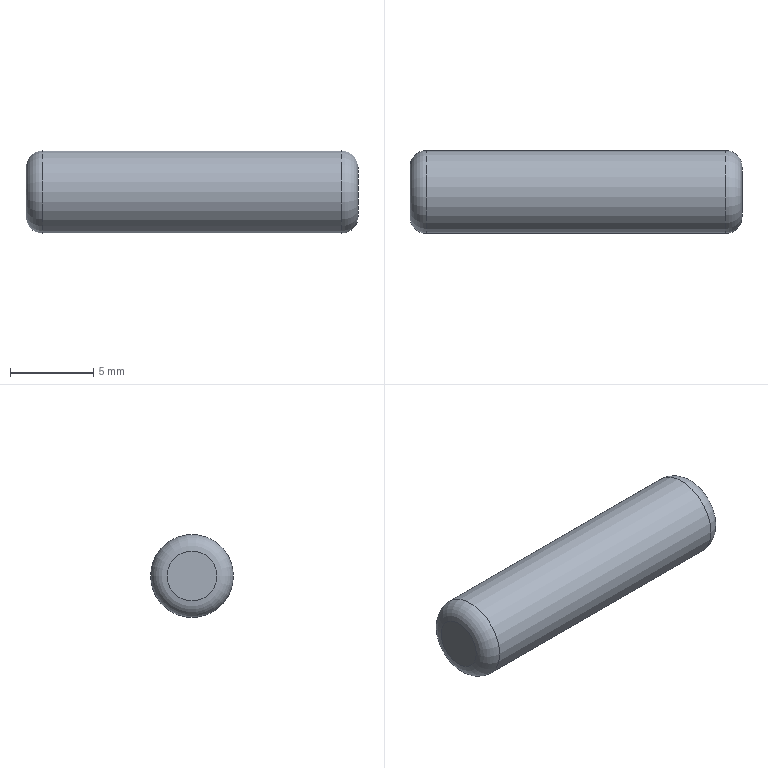Part | STEP file | 200 mesh_id630_x | 1 solid | 5 faces | box 20 x 5 x 5 mm | volume 386.56 mm3 | plane 2 | torus 2 | cylinder 1 | commonest cylinder face diameters 5 x1
STEP:
#1=CARTESIAN_POINT('',(-16706.684,-3961.269,27.6));
#2=VERTEX_POINT('',#1);
#3=CARTESIAN_POINT('',(-16706.684,-3962.769,27.6));
#4=DIRECTION('',(1.,0.,0.));
#5=DIRECTION('',(0.,1.,0.));
#6=AXIS2_PLACEMENT_3D('',#3,#4,#5);
#7=CIRCLE('',#6,1.5);
#8=EDGE_CURVE('',#2,#2,#7,.T.);
#9=ORIENTED_EDGE('',*,*,#8,.T.);
#10=EDGE_LOOP('',(#9));
#11=FACE_OUTER_BOUND('',#10,.T.);
#12=CARTESIAN_POINT('',(-16706.684,-3962.769,27.6));
#13=DIRECTION('',(1.,0.,0.));
#14=DIRECTION('',(0.,1.,0.));
#15=AXIS2_PLACEMENT_3D('',#12,#13,#14);
#16=PLANE('',#15);
#17=ADVANCED_FACE('',(#11),#16,.T.);
#18=CARTESIAN_POINT('',(-16726.684,-3964.269,27.6));
#19=VERTEX_POINT('',#18);
#20=CARTESIAN_POINT('',(-16726.684,-3962.769,27.6));
#21=DIRECTION('',(-1.,0.,0.));
#22=DIRECTION('',(0.,-1.,0.));
#23=AXIS2_PLACEMENT_3D('',#20,#21,#22);
#24=CIRCLE('',#23,1.5);
#25=EDGE_CURVE('',#19,#19,#24,.T.);
#26=ORIENTED_EDGE('',*,*,#25,.T.);
#27=EDGE_LOOP('',(#26));
#28=FACE_OUTER_BOUND('',#27,.T.);
#29=CARTESIAN_POINT('',(-16726.684,-3962.769,27.6));
#30=DIRECTION('',(-1.,0.,0.));
#31=DIRECTION('',(0.,-1.,0.));
#32=AXIS2_PLACEMENT_3D('',#29,#30,#31);
#33=PLANE('',#32);
#34=ADVANCED_FACE('',(#28),#33,.T.);
#35=CARTESIAN_POINT('',(-16707.684,-3960.269,27.6));
#36=VERTEX_POINT('',#35);
#37=CARTESIAN_POINT('',(-16707.684,-3962.769,27.6));
#38=DIRECTION('',(-1.,0.,0.));
#39=DIRECTION('',(0.,1.,0.));
#40=AXIS2_PLACEMENT_3D('',#37,#38,#39);
#41=CIRCLE('',#40,2.5);
#42=EDGE_CURVE('',#36,#36,#41,.T.);
#43=ORIENTED_EDGE('',*,*,#42,.T.);
#44=EDGE_LOOP('',(#43));
#45=FACE_BOUND('',#44,.T.);
#46=CARTESIAN_POINT('',(-16725.684,-3965.269,27.6));
#47=VERTEX_POINT('',#46);
#48=CARTESIAN_POINT('',(-16725.684,-3962.769,27.6));
#49=DIRECTION('',(1.,0.,0.));
#50=DIRECTION('',(0.,-1.,0.));
#51=AXIS2_PLACEMENT_3D('',#48,#49,#50);
#52=CIRCLE('',#51,2.5);
#53=EDGE_CURVE('',#47,#47,#52,.T.);
#54=ORIENTED_EDGE('',*,*,#53,.T.);
#55=EDGE_LOOP('',(#54));
#56=FACE_BOUND('',#55,.T.);
#57=CARTESIAN_POINT('',(-16721.684,-3962.769,27.6));
#58=DIRECTION('',(1.,0.,0.));
#59=DIRECTION('',(0.,0.,-1.));
#60=AXIS2_PLACEMENT_3D('',#57,#58,#59);
#61=CYLINDRICAL_SURFACE('',#60,2.5);
#62=ADVANCED_FACE('',(#45,#56),#61,.T.);
#63=ORIENTED_EDGE('',*,*,#8,.F.);
#64=EDGE_LOOP('',(#63));
#65=FACE_BOUND('',#64,.T.);
#66=ORIENTED_EDGE('',*,*,#42,.F.);
#67=EDGE_LOOP('',(#66));
#68=FACE_BOUND('',#67,.T.);
#69=CARTESIAN_POINT('',(-16707.684,-3962.769,27.6));
#70=DIRECTION('',(1.,0.,0.));
#71=DIRECTION('',(0.,1.,0.));
#72=AXIS2_PLACEMENT_3D('',#69,#70,#71);
#73=TOROIDAL_SURFACE('',#72,1.5,1.);
#74=ADVANCED_FACE('',(#65,#68),#73,.T.);
#75=ORIENTED_EDGE('',*,*,#25,.F.);
#76=EDGE_LOOP('',(#75));
#77=FACE_BOUND('',#76,.T.);
#78=ORIENTED_EDGE('',*,*,#53,.F.);
#79=EDGE_LOOP('',(#78));
#80=FACE_BOUND('',#79,.T.);
#81=CARTESIAN_POINT('',(-16725.684,-3962.769,27.6));
#82=DIRECTION('',(-1.,0.,0.));
#83=DIRECTION('',(0.,-1.,0.));
#84=AXIS2_PLACEMENT_3D('',#81,#82,#83);
#85=TOROIDAL_SURFACE('',#84,1.5,1.);
#86=ADVANCED_FACE('',(#77,#80),#85,.T.);
#87=CLOSED_SHELL('',(#17,#34,#62,#74,#86));
#88=MANIFOLD_SOLID_BREP('',#87);
#89=(LENGTH_UNIT()NAMED_UNIT(*)SI_UNIT(.MILLI.,.METRE.));
#90=UNCERTAINTY_MEASURE_WITH_UNIT(LENGTH_MEASURE(0.00002),#89,'','');
#91=(NAMED_UNIT(*)PLANE_ANGLE_UNIT()SI_UNIT($,.RADIAN.));
#92=PLANE_ANGLE_MEASURE_WITH_UNIT(PLANE_ANGLE_MEASURE(0.01745),#91);
#93=DIMENSIONAL_EXPONENTS(0.,0.,0.,0.,0.,0.,0.);
#94=(CONVERSION_BASED_UNIT('DEGREE',#92)NAMED_UNIT(#93)PLANE_ANGLE_UNIT());
#95=(NAMED_UNIT(*)SI_UNIT($,.STERADIAN.)SOLID_ANGLE_UNIT());
#96=(GEOMETRIC_REPRESENTATION_CONTEXT(3)GLOBAL_UNCERTAINTY_ASSIGNED_CONTEXT((#90))GLOBAL_UNIT_ASSIGNED_CONTEXT((#89,#94,#95))REPRESENTATION_CONTEXT('',''));
#97=ADVANCED_BREP_SHAPE_REPRESENTATION('',(#88),#96);